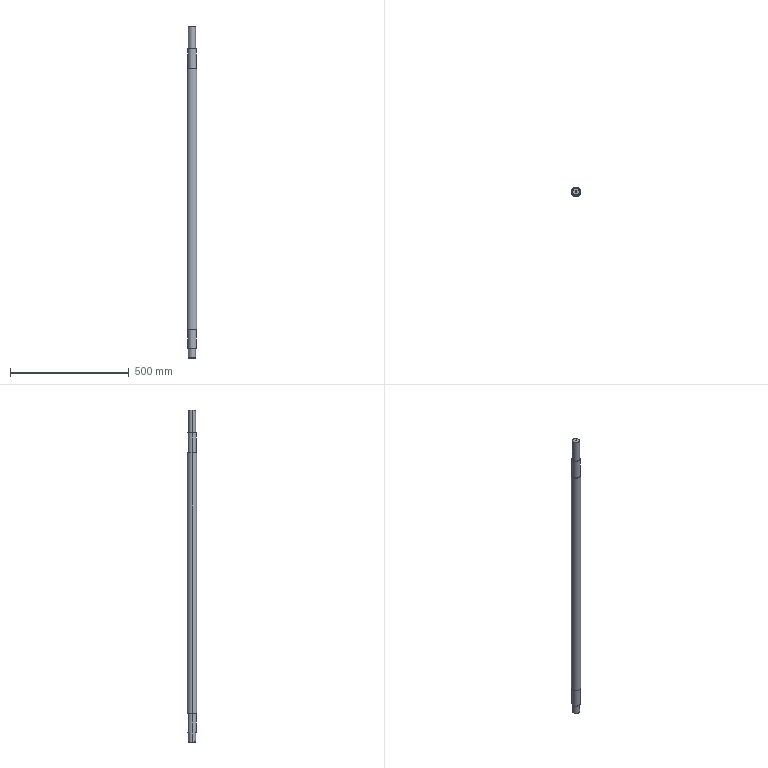Part | SolidWorks | features ICE 6, Chamfer 4, 3DProfileFeature 1, Extrusion 1, HoleWzd 1, MoveCopyBody 1 | 1 solid | 37 faces | box 40 x 40 x 1400 mm | volume 1632189 mm3 | cylinder 17 | cone 10 | plane 10 | commonest cylinder face diameters 30 x4 35 x4 8 x3 6.8 x2 26 x2 40 x2
STEP:
#1=CARTESIAN_POINT('',(0.,15.,-81.));
#2=VERTEX_POINT('',#1);
#3=CARTESIAN_POINT('',(4.,14.457,-77.));
#4=VERTEX_POINT('',#3);
#5=CARTESIAN_POINT('',(0.,15.,-81.));
#6=CARTESIAN_POINT('',(0.262,15.,-81.));
#7=CARTESIAN_POINT('',(0.5282,14.993,-80.974));
#8=CARTESIAN_POINT('',(1.042,14.966,-80.871));
#9=CARTESIAN_POINT('',(1.292,14.946,-80.795));
#10=CARTESIAN_POINT('',(2.02,14.871,-80.492));
#11=CARTESIAN_POINT('',(2.459,14.802,-80.198));
#12=CARTESIAN_POINT('',(3.014,14.695,-79.643));
#13=CARTESIAN_POINT('',(3.178,14.66,-79.443));
#14=CARTESIAN_POINT('',(3.467,14.594,-79.011));
#15=CARTESIAN_POINT('',(3.593,14.564,-78.777));
#16=CARTESIAN_POINT('',(3.794,14.513,-78.295));
#17=CARTESIAN_POINT('',(3.87,14.492,-78.046));
#18=CARTESIAN_POINT('',(3.973,14.464,-77.531));
#19=CARTESIAN_POINT('',(4.,14.457,-77.265));
#20=CARTESIAN_POINT('',(4.,14.457,-77.));
#21=B_SPLINE_CURVE_WITH_KNOTS('',3,(#5,#6,#7,#8,#9,#10,#11,#12,#13,#14,#15,#16,#17,#18,#19,#20),.UNSPECIFIED.,.F.,.F.,(4,2,2,2,2,2,2,4),(0.006283,0.007068,0.007852,0.009421,0.01021,0.01099,0.01177,0.01256),.UNSPECIFIED.);
#22=EDGE_CURVE('',#2,#4,#21,.T.);
#23=ORIENTED_EDGE('',*,*,#22,.F.);
#24=CARTESIAN_POINT('',(0.,11.,-81.));
#25=VERTEX_POINT('',#24);
#26=CARTESIAN_POINT('',(0.,20.,-81.));
#27=DIRECTION('',(0.,-1.,0.));
#28=VECTOR('',#27,1000.);
#29=LINE('',#26,#28);
#30=EDGE_CURVE('',#2,#25,#29,.T.);
#31=ORIENTED_EDGE('',*,*,#30,.T.);
#32=CARTESIAN_POINT('',(4.,11.,-77.));
#33=VERTEX_POINT('',#32);
#34=CARTESIAN_POINT('',(0.,11.,-77.));
#35=DIRECTION('',(0.,1.,0.));
#36=DIRECTION('',(0.,0.,1.));
#37=AXIS2_PLACEMENT_3D('',#34,#35,#36);
#38=CIRCLE('',#37,4.);
#39=EDGE_CURVE('',#33,#25,#38,.T.);
#40=ORIENTED_EDGE('',*,*,#39,.F.);
#41=CARTESIAN_POINT('',(4.,20.,-77.));
#42=DIRECTION('',(0.,-1.,0.));
#43=VECTOR('',#42,1000.);
#44=LINE('',#41,#43);
#45=EDGE_CURVE('',#4,#33,#44,.T.);
#46=ORIENTED_EDGE('',*,*,#45,.F.);
#47=EDGE_LOOP('',(#23,#31,#40,#46));
#48=FACE_OUTER_BOUND('',#47,.T.);
#49=CARTESIAN_POINT('',(0.,20.,-77.));
#50=DIRECTION('',(0.,-1.,0.));
#51=DIRECTION('',(0.,0.,-1.));
#52=AXIS2_PLACEMENT_3D('',#49,#50,#51);
#53=CYLINDRICAL_SURFACE('',#52,4.);
#54=ADVANCED_FACE('',(#48),#53,.F.);
#55=CARTESIAN_POINT('',(-3.4,0.,-18.75));
#56=VERTEX_POINT('',#55);
#57=CARTESIAN_POINT('',(3.4,0.,-18.75));
#58=VERTEX_POINT('',#57);
#59=CARTESIAN_POINT('',(0.,0.,-18.75));
#60=DIRECTION('',(0.,0.,1.));
#61=DIRECTION('',(1.,0.,0.));
#62=AXIS2_PLACEMENT_3D('',#59,#60,#61);
#63=CIRCLE('',#62,3.4);
#64=EDGE_CURVE('',#56,#58,#63,.T.);
#65=ORIENTED_EDGE('',*,*,#64,.F.);
#66=CARTESIAN_POINT('',(-3.4,0.,10.));
#67=VERTEX_POINT('',#66);
#68=CARTESIAN_POINT('',(-3.4,0.,10.));
#69=DIRECTION('',(0.,0.,1.));
#70=VECTOR('',#69,1000.);
#71=LINE('',#68,#70);
#72=EDGE_CURVE('',#56,#67,#71,.T.);
#73=ORIENTED_EDGE('',*,*,#72,.T.);
#74=CARTESIAN_POINT('',(3.4,0.,10.));
#75=VERTEX_POINT('',#74);
#76=CARTESIAN_POINT('',(0.,0.,10.));
#77=DIRECTION('',(0.,0.,1.));
#78=DIRECTION('',(1.,0.,0.));
#79=AXIS2_PLACEMENT_3D('',#76,#77,#78);
#80=CIRCLE('',#79,3.4);
#81=EDGE_CURVE('',#67,#75,#80,.T.);
#82=ORIENTED_EDGE('',*,*,#81,.T.);
#83=CARTESIAN_POINT('',(3.4,0.,10.));
#84=DIRECTION('',(0.,0.,1.));
#85=VECTOR('',#84,1000.);
#86=LINE('',#83,#85);
#87=EDGE_CURVE('',#58,#75,#86,.T.);
#88=ORIENTED_EDGE('',*,*,#87,.F.);
#89=EDGE_LOOP('',(#65,#73,#82,#88));
#90=FACE_OUTER_BOUND('',#89,.T.);
#91=CARTESIAN_POINT('',(0.,0.,10.));
#92=DIRECTION('',(0.,0.,1.));
#93=DIRECTION('',(1.,0.,0.));
#94=AXIS2_PLACEMENT_3D('',#91,#92,#93);
#95=CYLINDRICAL_SURFACE('',#94,3.4);
#96=ADVANCED_FACE('',(#90),#95,.F.);
#97=CARTESIAN_POINT('',(0.,0.,-20.793));
#98=VERTEX_POINT('',#97);
#99=CARTESIAN_POINT('',(3.4,0.,-18.75));
#100=DIRECTION('',(0.8572,0.,0.515));
#101=VECTOR('',#100,1000.);
#102=LINE('',#99,#101);
#103=EDGE_CURVE('',#98,#58,#102,.T.);
#104=ORIENTED_EDGE('',*,*,#103,.F.);
#105=CARTESIAN_POINT('',(-3.4,0.,-18.75));
#106=DIRECTION('',(-0.8572,0.,0.515));
#107=VECTOR('',#106,1000.);
#108=LINE('',#105,#107);
#109=EDGE_CURVE('',#98,#56,#108,.T.);
#110=ORIENTED_EDGE('',*,*,#109,.T.);
#111=ORIENTED_EDGE('',*,*,#64,.T.);
#112=EDGE_LOOP('',(#104,#110,#111));
#113=FACE_OUTER_BOUND('',#112,.T.);
#114=CARTESIAN_POINT('',(0.,0.,-18.75));
#115=DIRECTION('',(0.,0.,1.));
#116=DIRECTION('',(1.,0.,0.));
#117=AXIS2_PLACEMENT_3D('',#114,#115,#116);
#118=CONICAL_SURFACE('',#117,3.4,1.03);
#119=ADVANCED_FACE('',(#113),#118,.F.);
#120=CARTESIAN_POINT('',(14.,0.,10.));
#121=VERTEX_POINT('',#120);
#122=CARTESIAN_POINT('',(-14.,0.,10.));
#123=VERTEX_POINT('',#122);
#124=CARTESIAN_POINT('',(0.,0.,10.));
#125=DIRECTION('',(0.,0.,1.));
#126=DIRECTION('',(1.,0.,0.));
#127=AXIS2_PLACEMENT_3D('',#124,#125,#126);
#128=CIRCLE('',#127,14.);
#129=EDGE_CURVE('',#121,#123,#128,.T.);
#130=ORIENTED_EDGE('',*,*,#129,.F.);
#131=CARTESIAN_POINT('',(15.,0.,9.));
#132=VERTEX_POINT('',#131);
#133=CARTESIAN_POINT('',(14.,0.,10.));
#134=DIRECTION('',(0.7071,0.,-0.7071));
#135=VECTOR('',#134,1000.);
#136=LINE('',#133,#135);
#137=EDGE_CURVE('',#121,#132,#136,.T.);
#138=ORIENTED_EDGE('',*,*,#137,.T.);
#139=CARTESIAN_POINT('',(-15.,0.,9.));
#140=VERTEX_POINT('',#139);
#141=CARTESIAN_POINT('',(0.,0.,9.));
#142=DIRECTION('',(0.,0.,-1.));
#143=DIRECTION('',(1.,0.,0.));
#144=AXIS2_PLACEMENT_3D('',#141,#142,#143);
#145=CIRCLE('',#144,15.);
#146=EDGE_CURVE('',#140,#132,#145,.T.);
#147=ORIENTED_EDGE('',*,*,#146,.F.);
#148=CARTESIAN_POINT('',(-14.,0.,10.));
#149=DIRECTION('',(-0.7071,0.,-0.7071));
#150=VECTOR('',#149,1000.);
#151=LINE('',#148,#150);
#152=EDGE_CURVE('',#123,#140,#151,.T.);
#153=ORIENTED_EDGE('',*,*,#152,.F.);
#154=EDGE_LOOP('',(#130,#138,#147,#153));
#155=FACE_OUTER_BOUND('',#154,.T.);
#156=CARTESIAN_POINT('',(0.,0.,10.));
#157=DIRECTION('',(0.,0.,-1.));
#158=DIRECTION('',(-1.,0.,0.));
#159=AXIS2_PLACEMENT_3D('',#156,#157,#158);
#160=CONICAL_SURFACE('',#159,14.,0.7854);
#161=ADVANCED_FACE('',(#155),#160,.T.);
#162=CARTESIAN_POINT('',(19.,0.,-170.));
#163=VERTEX_POINT('',#162);
#164=CARTESIAN_POINT('',(-19.,0.,-170.));
#165=VERTEX_POINT('',#164);
#166=CARTESIAN_POINT('',(0.,0.,-170.));
#167=DIRECTION('',(0.,0.,1.));
#168=DIRECTION('',(-1.,0.,0.));
#169=AXIS2_PLACEMENT_3D('',#166,#167,#168);
#170=CIRCLE('',#169,19.);
#171=EDGE_CURVE('',#163,#165,#170,.T.);
#172=ORIENTED_EDGE('',*,*,#171,.F.);
#173=CARTESIAN_POINT('',(20.,0.,-171.));
#174=VERTEX_POINT('',#173);
#175=CARTESIAN_POINT('',(20.,0.,-171.));
#176=DIRECTION('',(0.7071,0.,-0.7071));
#177=VECTOR('',#176,1000.);
#178=LINE('',#175,#177);
#179=EDGE_CURVE('',#163,#174,#178,.T.);
#180=ORIENTED_EDGE('',*,*,#179,.T.);
#181=CARTESIAN_POINT('',(-20.,0.,-171.));
#182=VERTEX_POINT('',#181);
#183=CARTESIAN_POINT('',(0.,0.,-171.));
#184=DIRECTION('',(0.,0.,-1.));
#185=DIRECTION('',(-1.,0.,0.));
#186=AXIS2_PLACEMENT_3D('',#183,#184,#185);
#187=CIRCLE('',#186,20.);
#188=EDGE_CURVE('',#182,#174,#187,.T.);
#189=ORIENTED_EDGE('',*,*,#188,.F.);
#190=CARTESIAN_POINT('',(-20.,0.,-171.));
#191=DIRECTION('',(-0.7071,0.,-0.7071));
#192=VECTOR('',#191,1000.);
#193=LINE('',#190,#192);
#194=EDGE_CURVE('',#165,#182,#193,.T.);
#195=ORIENTED_EDGE('',*,*,#194,.F.);
#196=EDGE_LOOP('',(#172,#180,#189,#195));
#197=FACE_OUTER_BOUND('',#196,.T.);
#198=CARTESIAN_POINT('',(0.,0.,-171.));
#199=DIRECTION('',(0.,0.,-1.));
#200=DIRECTION('',(-1.,0.,0.));
#201=AXIS2_PLACEMENT_3D('',#198,#199,#200);
#202=CONICAL_SURFACE('',#201,20.,0.7854);
#203=ADVANCED_FACE('',(#197),#202,.T.);
#204=CARTESIAN_POINT('',(-19.,0.,-1270.));
#205=VERTEX_POINT('',#204);
#206=CARTESIAN_POINT('',(19.,0.,-1270.));
#207=VERTEX_POINT('',#206);
#208=CARTESIAN_POINT('',(0.,0.,-1270.));
#209=DIRECTION('',(0.,0.,-1.));
#210=DIRECTION('',(-1.,0.,0.));
#211=AXIS2_PLACEMENT_3D('',#208,#209,#210);
#212=CIRCLE('',#211,19.);
#213=EDGE_CURVE('',#205,#207,#212,.T.);
#214=ORIENTED_EDGE('',*,*,#213,.F.);
#215=CARTESIAN_POINT('',(-20.,0.,-1269.));
#216=VERTEX_POINT('',#215);
#217=CARTESIAN_POINT('',(-19.,0.,-1270.));
#218=DIRECTION('',(-0.7071,0.,0.7071));
#219=VECTOR('',#218,1000.);
#220=LINE('',#217,#219);
#221=EDGE_CURVE('',#205,#216,#220,.T.);
#222=ORIENTED_EDGE('',*,*,#221,.T.);
#223=CARTESIAN_POINT('',(20.,0.,-1269.));
#224=VERTEX_POINT('',#223);
#225=CARTESIAN_POINT('',(0.,0.,-1269.));
#226=DIRECTION('',(0.,0.,1.));
#227=DIRECTION('',(-1.,0.,0.));
#228=AXIS2_PLACEMENT_3D('',#225,#226,#227);
#229=CIRCLE('',#228,20.);
#230=EDGE_CURVE('',#224,#216,#229,.T.);
#231=ORIENTED_EDGE('',*,*,#230,.F.);
#232=CARTESIAN_POINT('',(19.,0.,-1270.));
#233=DIRECTION('',(0.7071,0.,0.7071));
#234=VECTOR('',#233,1000.);
#235=LINE('',#232,#234);
#236=EDGE_CURVE('',#207,#224,#235,.T.);
#237=ORIENTED_EDGE('',*,*,#236,.F.);
#238=EDGE_LOOP('',(#214,#222,#231,#237));
#239=FACE_OUTER_BOUND('',#238,.T.);
#240=CARTESIAN_POINT('',(0.,0.,-1270.));
#241=DIRECTION('',(0.,0.,1.));
#242=DIRECTION('',(1.,0.,0.));
#243=AXIS2_PLACEMENT_3D('',#240,#241,#242);
#244=CONICAL_SURFACE('',#243,19.,0.7854);
#245=ADVANCED_FACE('',(#239),#244,.T.);
#246=CARTESIAN_POINT('',(-14.,0.,-1390.));
#247=VERTEX_POINT('',#246);
#248=CARTESIAN_POINT('',(14.,0.,-1390.));
#249=VERTEX_POINT('',#248);
#250=CARTESIAN_POINT('',(0.,0.,-1390.));
#251=DIRECTION('',(0.,0.,-1.));
#252=DIRECTION('',(-1.,0.,0.));
#253=AXIS2_PLACEMENT_3D('',#250,#251,#252);
#254=CIRCLE('',#253,14.);
#255=EDGE_CURVE('',#247,#249,#254,.T.);
#256=ORIENTED_EDGE('',*,*,#255,.F.);
#257=CARTESIAN_POINT('',(-15.,0.,-1389.));
#258=VERTEX_POINT('',#257);
#259=CARTESIAN_POINT('',(-14.,0.,-1390.));
#260=DIRECTION('',(-0.7071,0.,0.7071));
#261=VECTOR('',#260,1000.);
#262=LINE('',#259,#261);
#263=EDGE_CURVE('',#247,#258,#262,.T.);
#264=ORIENTED_EDGE('',*,*,#263,.T.);
#265=CARTESIAN_POINT('',(15.,0.,-1389.));
#266=VERTEX_POINT('',#265);
#267=CARTESIAN_POINT('',(0.,0.,-1389.));
#268=DIRECTION('',(0.,0.,1.));
#269=DIRECTION('',(-1.,0.,0.));
#270=AXIS2_PLACEMENT_3D('',#267,#268,#269);
#271=CIRCLE('',#270,15.);
#272=EDGE_CURVE('',#266,#258,#271,.T.);
#273=ORIENTED_EDGE('',*,*,#272,.F.);
#274=CARTESIAN_POINT('',(14.,0.,-1390.));
#275=DIRECTION('',(0.7071,0.,0.7071));
#276=VECTOR('',#275,1000.);
#277=LINE('',#274,#276);
#278=EDGE_CURVE('',#249,#266,#277,.T.);
#279=ORIENTED_EDGE('',*,*,#278,.F.);
#280=EDGE_LOOP('',(#256,#264,#273,#279));
#281=FACE_OUTER_BOUND('',#280,.T.);
#282=CARTESIAN_POINT('',(0.,0.,-1390.));
#283=DIRECTION('',(0.,0.,1.));
#284=DIRECTION('',(1.,0.,0.));
#285=AXIS2_PLACEMENT_3D('',#282,#283,#284);
#286=CONICAL_SURFACE('',#285,14.,0.7854);
#287=ADVANCED_FACE('',(#281),#286,.T.);
#288=ORIENTED_EDGE('',*,*,#272,.T.);
#289=CARTESIAN_POINT('',(-15.,0.,-1352.));
#290=VERTEX_POINT('',#289);
#291=CARTESIAN_POINT('',(-15.,0.,-1390.));
#292=DIRECTION('',(0.,0.,1.));
#293=VECTOR('',#292,1000.);
#294=LINE('',#291,#293);
#295=EDGE_CURVE('',#258,#290,#294,.T.);
#296=ORIENTED_EDGE('',*,*,#295,.T.);
#297=CARTESIAN_POINT('',(15.,0.,-1352.));
#298=VERTEX_POINT('',#297);
#299=CARTESIAN_POINT('',(0.,0.,-1352.));
#300=DIRECTION('',(0.,0.,-1.));
#301=DIRECTION('',(-1.,0.,0.));
#302=AXIS2_PLACEMENT_3D('',#299,#300,#301);
#303=CIRCLE('',#302,15.);
#304=EDGE_CURVE('',#290,#298,#303,.T.);
#305=ORIENTED_EDGE('',*,*,#304,.T.);
#306=CARTESIAN_POINT('',(15.,0.,-1390.));
#307=DIRECTION('',(0.,0.,1.));
#308=VECTOR('',#307,1000.);
#309=LINE('',#306,#308);
#310=EDGE_CURVE('',#266,#298,#309,.T.);
#311=ORIENTED_EDGE('',*,*,#310,.F.);
#312=EDGE_LOOP('',(#288,#296,#305,#311));
#313=FACE_OUTER_BOUND('',#312,.T.);
#314=CARTESIAN_POINT('',(0.,0.,-1390.));
#315=DIRECTION('',(0.,0.,1.));
#316=DIRECTION('',(1.,0.,0.));
#317=AXIS2_PLACEMENT_3D('',#314,#315,#316);
#318=CYLINDRICAL_SURFACE('',#317,15.);
#319=ADVANCED_FACE('',(#313),#318,.T.);
#320=CARTESIAN_POINT('',(-13.,0.,-1352.));
#321=VERTEX_POINT('',#320);
#322=CARTESIAN_POINT('',(13.,0.,-1352.));
#323=VERTEX_POINT('',#322);
#324=CARTESIAN_POINT('',(0.,0.,-1352.));
#325=DIRECTION('',(0.,0.,-1.));
#326=DIRECTION('',(-1.,0.,0.));
#327=AXIS2_PLACEMENT_3D('',#324,#325,#326);
#328=CIRCLE('',#327,13.);
#329=EDGE_CURVE('',#321,#323,#328,.T.);
#330=ORIENTED_EDGE('',*,*,#329,.F.);
#331=CARTESIAN_POINT('',(-13.,0.,-1350.));
#332=VERTEX_POINT('',#331);
#333=CARTESIAN_POINT('',(-13.,0.,-1352.));
#334=DIRECTION('',(0.,0.,1.));
#335=VECTOR('',#334,1000.);
#336=LINE('',#333,#335);
#337=EDGE_CURVE('',#321,#332,#336,.T.);
#338=ORIENTED_EDGE('',*,*,#337,.T.);
#339=CARTESIAN_POINT('',(13.,0.,-1350.));
#340=VERTEX_POINT('',#339);
#341=CARTESIAN_POINT('',(0.,0.,-1350.));
#342=DIRECTION('',(0.,0.,-1.));
#343=DIRECTION('',(-1.,0.,0.));
#344=AXIS2_PLACEMENT_3D('',#341,#342,#343);
#345=CIRCLE('',#344,13.);
#346=EDGE_CURVE('',#332,#340,#345,.T.);
#347=ORIENTED_EDGE('',*,*,#346,.T.);
#348=CARTESIAN_POINT('',(13.,0.,-1352.));
#349=DIRECTION('',(0.,0.,1.));
#350=VECTOR('',#349,1000.);
#351=LINE('',#348,#350);
#352=EDGE_CURVE('',#323,#340,#351,.T.);
#353=ORIENTED_EDGE('',*,*,#352,.F.);
#354=EDGE_LOOP('',(#330,#338,#347,#353));
#355=FACE_OUTER_BOUND('',#354,.T.);
#356=CARTESIAN_POINT('',(0.,0.,-1352.));
#357=DIRECTION('',(0.,0.,1.));
#358=DIRECTION('',(1.,0.,0.));
#359=AXIS2_PLACEMENT_3D('',#356,#357,#358);
#360=CYLINDRICAL_SURFACE('',#359,13.);
#361=ADVANCED_FACE('',(#355),#360,.T.);
#362=CARTESIAN_POINT('',(-17.5,0.,-1350.));
#363=VERTEX_POINT('',#362);
#364=CARTESIAN_POINT('',(17.5,0.,-1350.));
#365=VERTEX_POINT('',#364);
#366=CARTESIAN_POINT('',(0.,0.,-1350.));
#367=DIRECTION('',(0.,0.,-1.));
#368=DIRECTION('',(-1.,0.,0.));
#369=AXIS2_PLACEMENT_3D('',#366,#367,#368);
#370=CIRCLE('',#369,17.5);
#371=EDGE_CURVE('',#363,#365,#370,.T.);
#372=ORIENTED_EDGE('',*,*,#371,.F.);
#373=CARTESIAN_POINT('',(-17.5,0.,-1270.));
#374=VERTEX_POINT('',#373);
#375=CARTESIAN_POINT('',(-17.5,0.,-1350.));
#376=DIRECTION('',(0.,0.,1.));
#377=VECTOR('',#376,1000.);
#378=LINE('',#375,#377);
#379=EDGE_CURVE('',#363,#374,#378,.T.);
#380=ORIENTED_EDGE('',*,*,#379,.T.);
#381=CARTESIAN_POINT('',(17.5,0.,-1270.));
#382=VERTEX_POINT('',#381);
#383=CARTESIAN_POINT('',(0.,0.,-1270.));
#384=DIRECTION('',(0.,0.,-1.));
#385=DIRECTION('',(-1.,0.,0.));
#386=AXIS2_PLACEMENT_3D('',#383,#384,#385);
#387=CIRCLE('',#386,17.5);
#388=EDGE_CURVE('',#374,#382,#387,.T.);
#389=ORIENTED_EDGE('',*,*,#388,.T.);
#390=CARTESIAN_POINT('',(17.5,0.,-1350.));
#391=DIRECTION('',(0.,0.,1.));
#392=VECTOR('',#391,1000.);
#393=LINE('',#390,#392);
#394=EDGE_CURVE('',#365,#382,#393,.T.);
#395=ORIENTED_EDGE('',*,*,#394,.F.);
#396=EDGE_LOOP('',(#372,#380,#389,#395));
#397=FACE_OUTER_BOUND('',#396,.T.);
#398=CARTESIAN_POINT('',(0.,0.,-1350.));
#399=DIRECTION('',(0.,0.,1.));
#400=DIRECTION('',(1.,0.,0.));
#401=AXIS2_PLACEMENT_3D('',#398,#399,#400);
#402=CYLINDRICAL_SURFACE('',#401,17.5);
#403=ADVANCED_FACE('',(#397),#402,.T.);
#404=ORIENTED_EDGE('',*,*,#230,.T.);
#405=CARTESIAN_POINT('',(-20.,0.,-1270.));
#406=DIRECTION('',(0.,0.,1.));
#407=VECTOR('',#406,1000.);
#408=LINE('',#405,#407);
#409=EDGE_CURVE('',#216,#182,#408,.T.);
#410=ORIENTED_EDGE('',*,*,#409,.T.);
#411=ORIENTED_EDGE('',*,*,#188,.T.);
#412=CARTESIAN_POINT('',(20.,0.,-1270.));
#413=DIRECTION('',(0.,0.,1.));
#414=VECTOR('',#413,1000.);
#415=LINE('',#412,#414);
#416=EDGE_CURVE('',#224,#174,#415,.T.);
#417=ORIENTED_EDGE('',*,*,#416,.F.);
#418=EDGE_LOOP('',(#404,#410,#411,#417));
#419=FACE_OUTER_BOUND('',#418,.T.);
#420=CARTESIAN_POINT('',(0.,0.,-1270.));
#421=DIRECTION('',(0.,0.,1.));
#422=DIRECTION('',(1.,0.,0.));
#423=AXIS2_PLACEMENT_3D('',#420,#421,#422);
#424=CYLINDRICAL_SURFACE('',#423,20.);
#425=ADVANCED_FACE('',(#419),#424,.T.);
#426=CARTESIAN_POINT('',(-17.5,0.,-170.));
#427=VERTEX_POINT('',#426);
#428=CARTESIAN_POINT('',(17.5,0.,-170.));
#429=VERTEX_POINT('',#428);
#430=CARTESIAN_POINT('',(0.,0.,-170.));
#431=DIRECTION('',(0.,0.,-1.));
#432=DIRECTION('',(-1.,0.,0.));
#433=AXIS2_PLACEMENT_3D('',#430,#431,#432);
#434=CIRCLE('',#433,17.5);
#435=EDGE_CURVE('',#427,#429,#434,.T.);
#436=ORIENTED_EDGE('',*,*,#435,.F.);
#437=CARTESIAN_POINT('',(-17.5,0.,-86.));
#438=VERTEX_POINT('',#437);
#439=CARTESIAN_POINT('',(-17.5,0.,-170.));
#440=DIRECTION('',(0.,0.,1.));
#441=VECTOR('',#440,1000.);
#442=LINE('',#439,#441);
#443=EDGE_CURVE('',#427,#438,#442,.T.);
#444=ORIENTED_EDGE('',*,*,#443,.T.);
#445=CARTESIAN_POINT('',(17.5,0.,-86.));
#446=VERTEX_POINT('',#445);
#447=CARTESIAN_POINT('',(0.,0.,-86.));
#448=DIRECTION('',(0.,0.,-1.));
#449=DIRECTION('',(-1.,0.,0.));
#450=AXIS2_PLACEMENT_3D('',#447,#448,#449);
#451=CIRCLE('',#450,17.5);
#452=EDGE_CURVE('',#438,#446,#451,.T.);
#453=ORIENTED_EDGE('',*,*,#452,.T.);
#454=CARTESIAN_POINT('',(17.5,0.,-170.));
#455=DIRECTION('',(0.,0.,1.));
#456=VECTOR('',#455,1000.);
#457=LINE('',#454,#456);
#458=EDGE_CURVE('',#429,#446,#457,.T.);
#459=ORIENTED_EDGE('',*,*,#458,.F.);
#460=EDGE_LOOP('',(#436,#444,#453,#459));
#461=FACE_OUTER_BOUND('',#460,.T.);
#462=CARTESIAN_POINT('',(0.,0.,-170.));
#463=DIRECTION('',(0.,0.,1.));
#464=DIRECTION('',(1.,0.,0.));
#465=AXIS2_PLACEMENT_3D('',#462,#463,#464);
#466=CYLINDRICAL_SURFACE('',#465,17.5);
#467=ADVANCED_FACE('',(#461),#466,.T.);
#468=CARTESIAN_POINT('',(-4.,14.457,-5.));
#469=VERTEX_POINT('',#468);
#470=CARTESIAN_POINT('',(-4.,14.457,-77.));
#471=VERTEX_POINT('',#470);
#472=CARTESIAN_POINT('',(-4.,14.457,-86.));
#473=DIRECTION('',(0.,0.,-1.));
#474=VECTOR('',#473,1000.);
#475=LINE('',#472,#474);
#476=EDGE_CURVE('',#469,#471,#475,.T.);
#477=ORIENTED_EDGE('',*,*,#476,.T.);
#478=CARTESIAN_POINT('',(-4.,14.457,-77.));
#479=CARTESIAN_POINT('',(-4.,14.457,-77.266));
#480=CARTESIAN_POINT('',(-3.974,14.464,-77.527));
#481=CARTESIAN_POINT('',(-3.871,14.492,-78.04));
#482=CARTESIAN_POINT('',(-3.794,14.513,-78.294));
#483=CARTESIAN_POINT('',(-3.593,14.564,-78.778));
#484=CARTESIAN_POINT('',(-3.47,14.594,-79.008));
#485=CARTESIAN_POINT('',(-3.179,14.66,-79.442));
#486=CARTESIAN_POINT('',(-3.011,14.696,-79.646));
#487=CARTESIAN_POINT('',(-2.644,14.766,-80.013));
#488=CARTESIAN_POINT('',(-2.443,14.801,-80.178));
#489=CARTESIAN_POINT('',(-2.006,14.867,-80.471));
#490=CARTESIAN_POINT('',(-1.775,14.897,-80.594));
#491=CARTESIAN_POINT('',(-1.293,14.946,-80.794));
#492=CARTESIAN_POINT('',(-1.04,14.966,-80.871));
#493=CARTESIAN_POINT('',(-0.5228,14.993,-80.974));
#494=CARTESIAN_POINT('',(-0.2623,15.,-81.));
#495=CARTESIAN_POINT('',(0.,15.,-81.));
#496=B_SPLINE_CURVE_WITH_KNOTS('',3,(#478,#479,#480,#481,#482,#483,#484,#485,#486,#487,#488,#489,#490,#491,#492,#493,#494,#495),.UNSPECIFIED.,.F.,.F.,(4,2,2,2,2,2,2,2,4),(0.,0.0007854,0.001571,0.002356,0.003142,0.003927,0.004712,0.005498,0.006283),.UNSPECIFIED.);
#497=EDGE_CURVE('',#471,#2,#496,.T.);
#498=ORIENTED_EDGE('',*,*,#497,.T.);
#499=ORIENTED_EDGE('',*,*,#22,.T.);
#500=CARTESIAN_POINT('',(4.,14.457,-5.));
#501=VERTEX_POINT('',#500);
#502=CARTESIAN_POINT('',(4.,14.457,-86.));
#503=DIRECTION('',(0.,0.,1.));
#504=VECTOR('',#503,1000.);
#505=LINE('',#502,#504);
#506=EDGE_CURVE('',#4,#501,#505,.T.);
#507=ORIENTED_EDGE('',*,*,#506,.T.);
#508=CARTESIAN_POINT('',(4.,14.457,-5.));
#509=CARTESIAN_POINT('',(4.,14.457,-4.734));
#510=CARTESIAN_POINT('',(3.974,14.464,-4.474));
#511=CARTESIAN_POINT('',(3.872,14.492,-3.961));
#512=CARTESIAN_POINT('',(3.794,14.513,-3.706));
#513=CARTESIAN_POINT('',(3.593,14.564,-3.223));
#514=CARTESIAN_POINT('',(3.47,14.594,-2.993));
#515=CARTESIAN_POINT('',(3.18,14.66,-2.56));
#516=CARTESIAN_POINT('',(3.012,14.696,-2.355));
#517=CARTESIAN_POINT('',(2.645,14.766,-1.988));
#518=CARTESIAN_POINT('',(2.444,14.801,-1.823));
#519=CARTESIAN_POINT('',(2.008,14.867,-1.53));
#520=CARTESIAN_POINT('',(1.777,14.896,-1.407));
#521=CARTESIAN_POINT('',(1.296,14.946,-1.207));
#522=CARTESIAN_POINT('',(1.043,14.966,-1.129));
#523=CARTESIAN_POINT('',(0.5261,14.993,-1.026));
#524=CARTESIAN_POINT('',(0.2658,15.,-1.));
#525=CARTESIAN_POINT('',(-0.2585,15.,-0.9998));
#526=CARTESIAN_POINT('',(-0.5249,14.993,-1.026));
#527=CARTESIAN_POINT('',(-1.039,14.966,-1.128));
#528=CARTESIAN_POINT('',(-1.289,14.947,-1.204));
#529=CARTESIAN_POINT('',(-2.017,14.872,-1.506));
#530=CARTESIAN_POINT('',(-2.457,14.802,-1.801));
#531=CARTESIAN_POINT('',(-3.012,14.696,-2.355));
#532=CARTESIAN_POINT('',(-3.177,14.66,-2.556));
#533=CARTESIAN_POINT('',(-3.467,14.595,-2.988));
#534=CARTESIAN_POINT('',(-3.593,14.564,-3.222));
#535=CARTESIAN_POINT('',(-3.793,14.513,-3.704));
#536=CARTESIAN_POINT('',(-3.87,14.492,-3.954));
#537=CARTESIAN_POINT('',(-3.973,14.464,-4.469));
#538=CARTESIAN_POINT('',(-4.,14.457,-4.734));
#539=CARTESIAN_POINT('',(-4.,14.457,-5.));
#540=B_SPLINE_CURVE_WITH_KNOTS('',3,(#508,#509,#510,#511,#512,#513,#514,#515,#516,#517,#518,#519,#520,#521,#522,#523,#524,#525,#526,#527,#528,#529,#530,#531,#532,#533,#534,#535,#536,#537,#538,#539),.UNSPECIFIED.,.F.,.F.,(4,2,2,2,2,2,2,2,2,2,2,2,2,2,2,4),(0.,0.0007849,0.00157,0.002355,0.00314,0.003925,0.00471,0.005494,0.006279,0.007064,0.007849,0.009419,0.0102,0.01099,0.01177,0.01256),.UNSPECIFIED.);
#541=EDGE_CURVE('',#501,#469,#540,.T.);
#542=ORIENTED_EDGE('',*,*,#541,.T.);
#543=EDGE_LOOP('',(#477,#498,#499,#507,#542));
#544=FACE_BOUND('',#543,.T.);
#545=CARTESIAN_POINT('',(15.,0.,-86.));
#546=VERTEX_POINT('',#545);
#547=CARTESIAN_POINT('',(-15.,0.,-86.));
#548=VERTEX_POINT('',#547);
#549=CARTESIAN_POINT('',(0.,0.,-86.));
#550=DIRECTION('',(0.,0.,1.));
#551=DIRECTION('',(-1.,0.,0.));
#552=AXIS2_PLACEMENT_3D('',#549,#550,#551);
#553=CIRCLE('',#552,15.);
#554=EDGE_CURVE('',#546,#548,#553,.T.);
#555=ORIENTED_EDGE('',*,*,#554,.T.);
#556=CARTESIAN_POINT('',(-15.,0.,-86.));
#557=DIRECTION('',(0.,0.,1.));
#558=VECTOR('',#557,1000.);
#559=LINE('',#556,#558);
#560=EDGE_CURVE('',#548,#140,#559,.T.);
#561=ORIENTED_EDGE('',*,*,#560,.T.);
#562=ORIENTED_EDGE('',*,*,#146,.T.);
#563=CARTESIAN_POINT('',(15.,0.,-86.));
#564=DIRECTION('',(0.,0.,1.));
#565=VECTOR('',#564,1000.);
#566=LINE('',#563,#565);
#567=EDGE_CURVE('',#546,#132,#566,.T.);
#568=ORIENTED_EDGE('',*,*,#567,.F.);
#569=EDGE_LOOP('',(#555,#561,#562,#568));
#570=FACE_OUTER_BOUND('',#569,.T.);
#571=CARTESIAN_POINT('',(0.,0.,-86.));
#572=DIRECTION('',(0.,0.,1.));
#573=DIRECTION('',(1.,0.,0.));
#574=AXIS2_PLACEMENT_3D('',#571,#572,#573);
#575=CYLINDRICAL_SURFACE('',#574,15.);
#576=ADVANCED_FACE('',(#544,#570),#575,.T.);
#577=ORIENTED_EDGE('',*,*,#560,.F.);
#578=CARTESIAN_POINT('',(0.,0.,-86.));
#579=DIRECTION('',(0.,0.,1.));
#580=DIRECTION('',(-1.,0.,0.));
#581=AXIS2_PLACEMENT_3D('',#578,#579,#580);
#582=CIRCLE('',#581,15.);
#583=EDGE_CURVE('',#548,#546,#582,.T.);
#584=ORIENTED_EDGE('',*,*,#583,.T.);
#585=ORIENTED_EDGE('',*,*,#567,.T.);
#586=CARTESIAN_POINT('',(0.,0.,9.));
#587=DIRECTION('',(0.,0.,-1.));
#588=DIRECTION('',(1.,0.,0.));
#589=AXIS2_PLACEMENT_3D('',#586,#587,#588);
#590=CIRCLE('',#589,15.);
#591=EDGE_CURVE('',#132,#140,#590,.T.);
#592=ORIENTED_EDGE('',*,*,#591,.T.);
#593=EDGE_LOOP('',(#577,#584,#585,#592));
#594=FACE_OUTER_BOUND('',#593,.T.);
#595=CARTESIAN_POINT('',(0.,0.,-86.));
#596=DIRECTION('',(0.,0.,1.));
#597=DIRECTION('',(1.,0.,0.));
#598=AXIS2_PLACEMENT_3D('',#595,#596,#597);
#599=CYLINDRICAL_SURFACE('',#598,15.);
#600=ADVANCED_FACE('',(#594),#599,.T.);
#601=CARTESIAN_POINT('',(0.,0.,-1350.));
#602=DIRECTION('',(0.,0.,-1.));
#603=DIRECTION('',(-1.,0.,0.));
#604=AXIS2_PLACEMENT_3D('',#601,#602,#603);
#605=CIRCLE('',#604,17.5);
#606=EDGE_CURVE('',#365,#363,#605,.T.);
#607=ORIENTED_EDGE('',*,*,#606,.T.);
#608=ORIENTED_EDGE('',*,*,#371,.T.);
#609=EDGE_LOOP('',(#607,#608));
#610=FACE_OUTER_BOUND('',#609,.T.);
#611=CARTESIAN_POINT('',(0.,0.,-1350.));
#612=DIRECTION('',(0.,0.,-1.));
#613=DIRECTION('',(-1.,0.,0.));
#614=AXIS2_PLACEMENT_3D('',#611,#612,#613);
#615=CIRCLE('',#614,13.);
#616=EDGE_CURVE('',#340,#332,#615,.T.);
#617=ORIENTED_EDGE('',*,*,#616,.F.);
#618=ORIENTED_EDGE('',*,*,#346,.F.);
#619=EDGE_LOOP('',(#617,#618));
#620=FACE_BOUND('',#619,.T.);
#621=CARTESIAN_POINT('',(0.,0.,-1350.));
#622=DIRECTION('',(0.,0.,-1.));
#623=DIRECTION('',(-1.,0.,0.));
#624=AXIS2_PLACEMENT_3D('',#621,#622,#623);
#625=PLANE('',#624);
#626=ADVANCED_FACE('',(#610,#620),#625,.T.);
#627=CARTESIAN_POINT('',(0.,0.,-1270.));
#628=DIRECTION('',(0.,0.,-1.));
#629=DIRECTION('',(-1.,0.,0.));
#630=AXIS2_PLACEMENT_3D('',#627,#628,#629);
#631=CIRCLE('',#630,19.);
#632=EDGE_CURVE('',#207,#205,#631,.T.);
#633=ORIENTED_EDGE('',*,*,#632,.T.);
#634=ORIENTED_EDGE('',*,*,#213,.T.);
#635=EDGE_LOOP('',(#633,#634));
#636=FACE_OUTER_BOUND('',#635,.T.);
#637=CARTESIAN_POINT('',(0.,0.,-1270.));
#638=DIRECTION('',(0.,0.,-1.));
#639=DIRECTION('',(-1.,0.,0.));
#640=AXIS2_PLACEMENT_3D('',#637,#638,#639);
#641=CIRCLE('',#640,17.5);
#642=EDGE_CURVE('',#382,#374,#641,.T.);
#643=ORIENTED_EDGE('',*,*,#642,.F.);
#644=ORIENTED_EDGE('',*,*,#388,.F.);
#645=EDGE_LOOP('',(#643,#644));
#646=FACE_BOUND('',#645,.T.);
#647=CARTESIAN_POINT('',(0.,0.,-1270.));
#648=DIRECTION('',(0.,0.,-1.));
#649=DIRECTION('',(-1.,0.,0.));
#650=AXIS2_PLACEMENT_3D('',#647,#648,#649);
#651=PLANE('',#650);
#652=ADVANCED_FACE('',(#636,#646),#651,.T.);
#653=CARTESIAN_POINT('',(0.,0.,10.));
#654=DIRECTION('',(0.,0.,1.));
#655=DIRECTION('',(1.,0.,0.));
#656=AXIS2_PLACEMENT_3D('',#653,#654,#655);
#657=CIRCLE('',#656,3.4);
#658=EDGE_CURVE('',#75,#67,#657,.T.);
#659=ORIENTED_EDGE('',*,*,#658,.F.);
#660=ORIENTED_EDGE('',*,*,#81,.F.);
#661=EDGE_LOOP('',(#659,#660));
#662=FACE_BOUND('',#661,.T.);
#663=CARTESIAN_POINT('',(0.,0.,10.));
#664=DIRECTION('',(0.,0.,1.));
#665=DIRECTION('',(1.,0.,0.));
#666=AXIS2_PLACEMENT_3D('',#663,#664,#665);
#667=CIRCLE('',#666,14.);
#668=EDGE_CURVE('',#123,#121,#667,.T.);
#669=ORIENTED_EDGE('',*,*,#668,.T.);
#670=ORIENTED_EDGE('',*,*,#129,.T.);
#671=EDGE_LOOP('',(#669,#670));
#672=FACE_OUTER_BOUND('',#671,.T.);
#673=CARTESIAN_POINT('',(0.,0.,10.));
#674=DIRECTION('',(0.,0.,1.));
#675=DIRECTION('',(1.,0.,0.));
#676=AXIS2_PLACEMENT_3D('',#673,#674,#675);
#677=PLANE('',#676);
#678=ADVANCED_FACE('',(#662,#672),#677,.T.);
#679=ORIENTED_EDGE('',*,*,#443,.F.);
#680=CARTESIAN_POINT('',(0.,0.,-170.));
#681=DIRECTION('',(0.,0.,-1.));
#682=DIRECTION('',(-1.,0.,0.));
#683=AXIS2_PLACEMENT_3D('',#680,#681,#682);
#684=CIRCLE('',#683,17.5);
#685=EDGE_CURVE('',#429,#427,#684,.T.);
#686=ORIENTED_EDGE('',*,*,#685,.F.);
#687=ORIENTED_EDGE('',*,*,#458,.T.);
#688=CARTESIAN_POINT('',(0.,0.,-86.));
#689=DIRECTION('',(0.,0.,-1.));
#690=DIRECTION('',(-1.,0.,0.));
#691=AXIS2_PLACEMENT_3D('',#688,#689,#690);
#692=CIRCLE('',#691,17.5);
#693=EDGE_CURVE('',#446,#438,#692,.T.);
#694=ORIENTED_EDGE('',*,*,#693,.T.);
#695=EDGE_LOOP('',(#679,#686,#687,#694));
#696=FACE_OUTER_BOUND('',#695,.T.);
#697=CARTESIAN_POINT('',(0.,0.,-170.));
#698=DIRECTION('',(0.,0.,1.));
#699=DIRECTION('',(1.,0.,0.));
#700=AXIS2_PLACEMENT_3D('',#697,#698,#699);
#701=CYLINDRICAL_SURFACE('',#700,17.5);
#702=ADVANCED_FACE('',(#696),#701,.T.);
#703=ORIENTED_EDGE('',*,*,#554,.F.);
#704=ORIENTED_EDGE('',*,*,#583,.F.);
#705=EDGE_LOOP('',(#703,#704));
#706=FACE_BOUND('',#705,.T.);
#707=ORIENTED_EDGE('',*,*,#693,.F.);
#708=ORIENTED_EDGE('',*,*,#452,.F.);
#709=EDGE_LOOP('',(#707,#708));
#710=FACE_OUTER_BOUND('',#709,.T.);
#711=CARTESIAN_POINT('',(0.,0.,-86.));
#712=DIRECTION('',(0.,0.,-1.));
#713=DIRECTION('',(-1.,0.,0.));
#714=AXIS2_PLACEMENT_3D('',#711,#712,#713);
#715=PLANE('',#714);
#716=ADVANCED_FACE('',(#706,#710),#715,.F.);
#717=CARTESIAN_POINT('',(0.,0.,-170.));
#718=DIRECTION('',(0.,0.,1.));
#719=DIRECTION('',(-1.,0.,0.));
#720=AXIS2_PLACEMENT_3D('',#717,#718,#719);
#721=CIRCLE('',#720,19.);
#722=EDGE_CURVE('',#165,#163,#721,.T.);
#723=ORIENTED_EDGE('',*,*,#722,.T.);
#724=ORIENTED_EDGE('',*,*,#171,.T.);
#725=EDGE_LOOP('',(#723,#724));
#726=FACE_OUTER_BOUND('',#725,.T.);
#727=ORIENTED_EDGE('',*,*,#685,.T.);
#728=ORIENTED_EDGE('',*,*,#435,.T.);
#729=EDGE_LOOP('',(#727,#728));
#730=FACE_BOUND('',#729,.T.);
#731=CARTESIAN_POINT('',(0.,0.,-170.));
#732=DIRECTION('',(0.,0.,-1.));
#733=DIRECTION('',(-1.,0.,0.));
#734=AXIS2_PLACEMENT_3D('',#731,#732,#733);
#735=PLANE('',#734);
#736=ADVANCED_FACE('',(#726,#730),#735,.F.);
#737=ORIENTED_EDGE('',*,*,#409,.F.);
#738=CARTESIAN_POINT('',(0.,0.,-1269.));
#739=DIRECTION('',(0.,0.,1.));
#740=DIRECTION('',(-1.,0.,0.));
#741=AXIS2_PLACEMENT_3D('',#738,#739,#740);
#742=CIRCLE('',#741,20.);
#743=EDGE_CURVE('',#216,#224,#742,.T.);
#744=ORIENTED_EDGE('',*,*,#743,.T.);
#745=ORIENTED_EDGE('',*,*,#416,.T.);
#746=CARTESIAN_POINT('',(0.,0.,-171.));
#747=DIRECTION('',(0.,0.,-1.));
#748=DIRECTION('',(-1.,0.,0.));
#749=AXIS2_PLACEMENT_3D('',#746,#747,#748);
#750=CIRCLE('',#749,20.);
#751=EDGE_CURVE('',#174,#182,#750,.T.);
#752=ORIENTED_EDGE('',*,*,#751,.T.);
#753=EDGE_LOOP('',(#737,#744,#745,#752));
#754=FACE_OUTER_BOUND('',#753,.T.);
#755=CARTESIAN_POINT('',(0.,0.,-1270.));
#756=DIRECTION('',(0.,0.,1.));
#757=DIRECTION('',(1.,0.,0.));
#758=AXIS2_PLACEMENT_3D('',#755,#756,#757);
#759=CYLINDRICAL_SURFACE('',#758,20.);
#760=ADVANCED_FACE('',(#754),#759,.T.);
#761=ORIENTED_EDGE('',*,*,#379,.F.);
#762=ORIENTED_EDGE('',*,*,#606,.F.);
#763=ORIENTED_EDGE('',*,*,#394,.T.);
#764=ORIENTED_EDGE('',*,*,#642,.T.);
#765=EDGE_LOOP('',(#761,#762,#763,#764));
#766=FACE_OUTER_BOUND('',#765,.T.);
#767=CARTESIAN_POINT('',(0.,0.,-1350.));
#768=DIRECTION('',(0.,0.,1.));
#769=DIRECTION('',(1.,0.,0.));
#770=AXIS2_PLACEMENT_3D('',#767,#768,#769);
#771=CYLINDRICAL_SURFACE('',#770,17.5);
#772=ADVANCED_FACE('',(#766),#771,.T.);
#773=ORIENTED_EDGE('',*,*,#337,.F.);
#774=CARTESIAN_POINT('',(0.,0.,-1352.));
#775=DIRECTION('',(0.,0.,-1.));
#776=DIRECTION('',(-1.,0.,0.));
#777=AXIS2_PLACEMENT_3D('',#774,#775,#776);
#778=CIRCLE('',#777,13.);
#779=EDGE_CURVE('',#323,#321,#778,.T.);
#780=ORIENTED_EDGE('',*,*,#779,.F.);
#781=ORIENTED_EDGE('',*,*,#352,.T.);
#782=ORIENTED_EDGE('',*,*,#616,.T.);
#783=EDGE_LOOP('',(#773,#780,#781,#782));
#784=FACE_OUTER_BOUND('',#783,.T.);
#785=CARTESIAN_POINT('',(0.,0.,-1352.));
#786=DIRECTION('',(0.,0.,1.));
#787=DIRECTION('',(1.,0.,0.));
#788=AXIS2_PLACEMENT_3D('',#785,#786,#787);
#789=CYLINDRICAL_SURFACE('',#788,13.);
#790=ADVANCED_FACE('',(#784),#789,.T.);
#791=CARTESIAN_POINT('',(0.,0.,-1352.));
#792=DIRECTION('',(0.,0.,-1.));
#793=DIRECTION('',(-1.,0.,0.));
#794=AXIS2_PLACEMENT_3D('',#791,#792,#793);
#795=CIRCLE('',#794,15.);
#796=EDGE_CURVE('',#298,#290,#795,.T.);
#797=ORIENTED_EDGE('',*,*,#796,.F.);
#798=ORIENTED_EDGE('',*,*,#304,.F.);
#799=EDGE_LOOP('',(#797,#798));
#800=FACE_OUTER_BOUND('',#799,.T.);
#801=ORIENTED_EDGE('',*,*,#779,.T.);
#802=ORIENTED_EDGE('',*,*,#329,.T.);
#803=EDGE_LOOP('',(#801,#802));
#804=FACE_BOUND('',#803,.T.);
#805=CARTESIAN_POINT('',(0.,0.,-1352.));
#806=DIRECTION('',(0.,0.,-1.));
#807=DIRECTION('',(-1.,0.,0.));
#808=AXIS2_PLACEMENT_3D('',#805,#806,#807);
#809=PLANE('',#808);
#810=ADVANCED_FACE('',(#800,#804),#809,.F.);
#811=ORIENTED_EDGE('',*,*,#295,.F.);
#812=CARTESIAN_POINT('',(0.,0.,-1389.));
#813=DIRECTION('',(0.,0.,1.));
#814=DIRECTION('',(-1.,0.,0.));
#815=AXIS2_PLACEMENT_3D('',#812,#813,#814);
#816=CIRCLE('',#815,15.);
#817=EDGE_CURVE('',#258,#266,#816,.T.);
#818=ORIENTED_EDGE('',*,*,#817,.T.);
#819=ORIENTED_EDGE('',*,*,#310,.T.);
#820=ORIENTED_EDGE('',*,*,#796,.T.);
#821=EDGE_LOOP('',(#811,#818,#819,#820));
#822=FACE_OUTER_BOUND('',#821,.T.);
#823=CARTESIAN_POINT('',(0.,0.,-1390.));
#824=DIRECTION('',(0.,0.,1.));
#825=DIRECTION('',(1.,0.,0.));
#826=AXIS2_PLACEMENT_3D('',#823,#824,#825);
#827=CYLINDRICAL_SURFACE('',#826,15.);
#828=ADVANCED_FACE('',(#822),#827,.T.);
#829=CARTESIAN_POINT('',(0.,0.,-1390.));
#830=DIRECTION('',(0.,0.,-1.));
#831=DIRECTION('',(-1.,0.,0.));
#832=AXIS2_PLACEMENT_3D('',#829,#830,#831);
#833=CIRCLE('',#832,14.);
#834=EDGE_CURVE('',#249,#247,#833,.T.);
#835=ORIENTED_EDGE('',*,*,#834,.T.);
#836=ORIENTED_EDGE('',*,*,#255,.T.);
#837=EDGE_LOOP('',(#835,#836));
#838=FACE_OUTER_BOUND('',#837,.T.);
#839=CARTESIAN_POINT('',(0.,0.,-1390.));
#840=DIRECTION('',(0.,0.,-1.));
#841=DIRECTION('',(-1.,0.,0.));
#842=AXIS2_PLACEMENT_3D('',#839,#840,#841);
#843=PLANE('',#842);
#844=ADVANCED_FACE('',(#838),#843,.T.);
#845=ORIENTED_EDGE('',*,*,#263,.F.);
#846=ORIENTED_EDGE('',*,*,#834,.F.);
#847=ORIENTED_EDGE('',*,*,#278,.T.);
#848=ORIENTED_EDGE('',*,*,#817,.F.);
#849=EDGE_LOOP('',(#845,#846,#847,#848));
#850=FACE_OUTER_BOUND('',#849,.T.);
#851=CARTESIAN_POINT('',(0.,0.,-1390.));
#852=DIRECTION('',(0.,0.,1.));
#853=DIRECTION('',(1.,0.,0.));
#854=AXIS2_PLACEMENT_3D('',#851,#852,#853);
#855=CONICAL_SURFACE('',#854,14.,0.7854);
#856=ADVANCED_FACE('',(#850),#855,.T.);
#857=ORIENTED_EDGE('',*,*,#221,.F.);
#858=ORIENTED_EDGE('',*,*,#632,.F.);
#859=ORIENTED_EDGE('',*,*,#236,.T.);
#860=ORIENTED_EDGE('',*,*,#743,.F.);
#861=EDGE_LOOP('',(#857,#858,#859,#860));
#862=FACE_OUTER_BOUND('',#861,.T.);
#863=CARTESIAN_POINT('',(0.,0.,-1270.));
#864=DIRECTION('',(0.,0.,1.));
#865=DIRECTION('',(1.,0.,0.));
#866=AXIS2_PLACEMENT_3D('',#863,#864,#865);
#867=CONICAL_SURFACE('',#866,19.,0.7854);
#868=ADVANCED_FACE('',(#862),#867,.T.);
#869=ORIENTED_EDGE('',*,*,#179,.F.);
#870=ORIENTED_EDGE('',*,*,#722,.F.);
#871=ORIENTED_EDGE('',*,*,#194,.T.);
#872=ORIENTED_EDGE('',*,*,#751,.F.);
#873=EDGE_LOOP('',(#869,#870,#871,#872));
#874=FACE_OUTER_BOUND('',#873,.T.);
#875=CARTESIAN_POINT('',(0.,0.,-171.));
#876=DIRECTION('',(0.,0.,-1.));
#877=DIRECTION('',(-1.,0.,0.));
#878=AXIS2_PLACEMENT_3D('',#875,#876,#877);
#879=CONICAL_SURFACE('',#878,20.,0.7854);
#880=ADVANCED_FACE('',(#874),#879,.T.);
#881=ORIENTED_EDGE('',*,*,#137,.F.);
#882=ORIENTED_EDGE('',*,*,#668,.F.);
#883=ORIENTED_EDGE('',*,*,#152,.T.);
#884=ORIENTED_EDGE('',*,*,#591,.F.);
#885=EDGE_LOOP('',(#881,#882,#883,#884));
#886=FACE_OUTER_BOUND('',#885,.T.);
#887=CARTESIAN_POINT('',(0.,0.,10.));
#888=DIRECTION('',(0.,0.,-1.));
#889=DIRECTION('',(-1.,0.,0.));
#890=AXIS2_PLACEMENT_3D('',#887,#888,#889);
#891=CONICAL_SURFACE('',#890,14.,0.7854);
#892=ADVANCED_FACE('',(#886),#891,.T.);
#893=ORIENTED_EDGE('',*,*,#109,.F.);
#894=ORIENTED_EDGE('',*,*,#103,.T.);
#895=CARTESIAN_POINT('',(0.,0.,-18.75));
#896=DIRECTION('',(0.,0.,1.));
#897=DIRECTION('',(1.,0.,0.));
#898=AXIS2_PLACEMENT_3D('',#895,#896,#897);
#899=CIRCLE('',#898,3.4);
#900=EDGE_CURVE('',#58,#56,#899,.T.);
#901=ORIENTED_EDGE('',*,*,#900,.T.);
#902=EDGE_LOOP('',(#893,#894,#901));
#903=FACE_OUTER_BOUND('',#902,.T.);
#904=CARTESIAN_POINT('',(0.,0.,-18.75));
#905=DIRECTION('',(0.,0.,1.));
#906=DIRECTION('',(1.,0.,0.));
#907=AXIS2_PLACEMENT_3D('',#904,#905,#906);
#908=CONICAL_SURFACE('',#907,3.4,1.03);
#909=ADVANCED_FACE('',(#903),#908,.F.);
#910=ORIENTED_EDGE('',*,*,#72,.F.);
#911=ORIENTED_EDGE('',*,*,#900,.F.);
#912=ORIENTED_EDGE('',*,*,#87,.T.);
#913=ORIENTED_EDGE('',*,*,#658,.T.);
#914=EDGE_LOOP('',(#910,#911,#912,#913));
#915=FACE_OUTER_BOUND('',#914,.T.);
#916=CARTESIAN_POINT('',(0.,0.,10.));
#917=DIRECTION('',(0.,0.,1.));
#918=DIRECTION('',(1.,0.,0.));
#919=AXIS2_PLACEMENT_3D('',#916,#917,#918);
#920=CYLINDRICAL_SURFACE('',#919,3.4);
#921=ADVANCED_FACE('',(#915),#920,.F.);
#922=ORIENTED_EDGE('',*,*,#30,.F.);
#923=ORIENTED_EDGE('',*,*,#497,.F.);
#924=CARTESIAN_POINT('',(-4.,11.,-77.));
#925=VERTEX_POINT('',#924);
#926=CARTESIAN_POINT('',(-4.,20.,-77.));
#927=DIRECTION('',(0.,-1.,0.));
#928=VECTOR('',#927,1000.);
#929=LINE('',#926,#928);
#930=EDGE_CURVE('',#471,#925,#929,.T.);
#931=ORIENTED_EDGE('',*,*,#930,.T.);
#932=CARTESIAN_POINT('',(0.,11.,-77.));
#933=DIRECTION('',(0.,1.,0.));
#934=DIRECTION('',(0.,0.,1.));
#935=AXIS2_PLACEMENT_3D('',#932,#933,#934);
#936=CIRCLE('',#935,4.);
#937=EDGE_CURVE('',#25,#925,#936,.T.);
#938=ORIENTED_EDGE('',*,*,#937,.F.);
#939=EDGE_LOOP('',(#922,#923,#931,#938));
#940=FACE_OUTER_BOUND('',#939,.T.);
#941=CARTESIAN_POINT('',(0.,20.,-77.));
#942=DIRECTION('',(0.,-1.,0.));
#943=DIRECTION('',(0.,0.,-1.));
#944=AXIS2_PLACEMENT_3D('',#941,#942,#943);
#945=CYLINDRICAL_SURFACE('',#944,4.);
#946=ADVANCED_FACE('',(#940),#945,.F.);
#947=CARTESIAN_POINT('',(-4.,11.,-5.));
#948=VERTEX_POINT('',#947);
#949=CARTESIAN_POINT('',(-4.,20.,-5.));
#950=DIRECTION('',(0.,-1.,0.));
#951=VECTOR('',#950,1000.);
#952=LINE('',#949,#951);
#953=EDGE_CURVE('',#469,#948,#952,.T.);
#954=ORIENTED_EDGE('',*,*,#953,.T.);
#955=CARTESIAN_POINT('',(-4.,11.,-77.));
#956=DIRECTION('',(0.,0.,1.));
#957=VECTOR('',#956,1000.);
#958=LINE('',#955,#957);
#959=EDGE_CURVE('',#925,#948,#958,.T.);
#960=ORIENTED_EDGE('',*,*,#959,.F.);
#961=ORIENTED_EDGE('',*,*,#930,.F.);
#962=ORIENTED_EDGE('',*,*,#476,.F.);
#963=EDGE_LOOP('',(#954,#960,#961,#962));
#964=FACE_OUTER_BOUND('',#963,.T.);
#965=CARTESIAN_POINT('',(-4.,20.,-77.));
#966=DIRECTION('',(1.,0.,0.));
#967=DIRECTION('',(0.,0.,-1.));
#968=AXIS2_PLACEMENT_3D('',#965,#966,#967);
#969=PLANE('',#968);
#970=ADVANCED_FACE('',(#964),#969,.T.);
#971=CARTESIAN_POINT('',(4.,11.,-5.));
#972=VERTEX_POINT('',#971);
#973=CARTESIAN_POINT('',(4.,20.,-5.));
#974=DIRECTION('',(0.,-1.,0.));
#975=VECTOR('',#974,1000.);
#976=LINE('',#973,#975);
#977=EDGE_CURVE('',#501,#972,#976,.T.);
#978=ORIENTED_EDGE('',*,*,#977,.T.);
#979=CARTESIAN_POINT('',(0.,11.,-5.));
#980=DIRECTION('',(0.,1.,0.));
#981=DIRECTION('',(0.,0.,1.));
#982=AXIS2_PLACEMENT_3D('',#979,#980,#981);
#983=CIRCLE('',#982,4.);
#984=EDGE_CURVE('',#948,#972,#983,.T.);
#985=ORIENTED_EDGE('',*,*,#984,.F.);
#986=ORIENTED_EDGE('',*,*,#953,.F.);
#987=ORIENTED_EDGE('',*,*,#541,.F.);
#988=EDGE_LOOP('',(#978,#985,#986,#987));
#989=FACE_OUTER_BOUND('',#988,.T.);
#990=CARTESIAN_POINT('',(0.,20.,-5.));
#991=DIRECTION('',(0.,-1.,0.));
#992=DIRECTION('',(0.,0.,-1.));
#993=AXIS2_PLACEMENT_3D('',#990,#991,#992);
#994=CYLINDRICAL_SURFACE('',#993,4.);
#995=ADVANCED_FACE('',(#989),#994,.F.);
#996=ORIENTED_EDGE('',*,*,#45,.T.);
#997=CARTESIAN_POINT('',(4.,11.,-77.));
#998=DIRECTION('',(0.,0.,-1.));
#999=VECTOR('',#998,1000.);
#1000=LINE('',#997,#999);
#1001=EDGE_CURVE('',#972,#33,#1000,.T.);
#1002=ORIENTED_EDGE('',*,*,#1001,.F.);
#1003=ORIENTED_EDGE('',*,*,#977,.F.);
#1004=ORIENTED_EDGE('',*,*,#506,.F.);
#1005=EDGE_LOOP('',(#996,#1002,#1003,#1004));
#1006=FACE_OUTER_BOUND('',#1005,.T.);
#1007=CARTESIAN_POINT('',(4.,20.,-77.));
#1008=DIRECTION('',(-1.,0.,0.));
#1009=DIRECTION('',(0.,0.,1.));
#1010=AXIS2_PLACEMENT_3D('',#1007,#1008,#1009);
#1011=PLANE('',#1010);
#1012=ADVANCED_FACE('',(#1006),#1011,.T.);
#1013=ORIENTED_EDGE('',*,*,#39,.T.);
#1014=ORIENTED_EDGE('',*,*,#937,.T.);
#1015=ORIENTED_EDGE('',*,*,#959,.T.);
#1016=ORIENTED_EDGE('',*,*,#984,.T.);
#1017=ORIENTED_EDGE('',*,*,#1001,.T.);
#1018=EDGE_LOOP('',(#1013,#1014,#1015,#1016,#1017));
#1019=FACE_OUTER_BOUND('',#1018,.T.);
#1020=CARTESIAN_POINT('',(0.,11.,-77.));
#1021=DIRECTION('',(0.,1.,0.));
#1022=DIRECTION('',(0.,0.,1.));
#1023=AXIS2_PLACEMENT_3D('',#1020,#1021,#1022);
#1024=PLANE('',#1023);
#1025=ADVANCED_FACE('',(#1019),#1024,.T.);
#1026=CLOSED_SHELL('',(#54,#96,#119,#161,#203,#245,#287,#319,#361,#403,#425,#467,#576,#600,#626,#652,#678,#702,#716,#736,#760,#772,#790,#810,#828,#844,#856,#868,#880,#892,#909,#921,#946,#970,#995,#1012,#1025));
#1027=MANIFOLD_SOLID_BREP('',#1026);
#1028=CARTESIAN_POINT('',(0.,0.,0.));
#1029=DIRECTION('',(0.,0.,1.));
#1030=DIRECTION('',(1.,0.,0.));
#1031=AXIS2_PLACEMENT_3D('',#1028,#1029,#1030);
#1032=(LENGTH_UNIT()NAMED_UNIT(*)SI_UNIT(.MILLI.,.METRE.));
#1033=UNCERTAINTY_MEASURE_WITH_UNIT(LENGTH_MEASURE(0.00001),#1032,'','');
#1034=(NAMED_UNIT(*)PLANE_ANGLE_UNIT()SI_UNIT($,.RADIAN.));
#1035=(NAMED_UNIT(*)SI_UNIT($,.STERADIAN.)SOLID_ANGLE_UNIT());
#1036=(GEOMETRIC_REPRESENTATION_CONTEXT(3)GLOBAL_UNCERTAINTY_ASSIGNED_CONTEXT((#1033))GLOBAL_UNIT_ASSIGNED_CONTEXT((#1032,#1034,#1035))REPRESENTATION_CONTEXT('',''));
#1037=ADVANCED_BREP_SHAPE_REPRESENTATION('',(#1027,#1031),#1036);